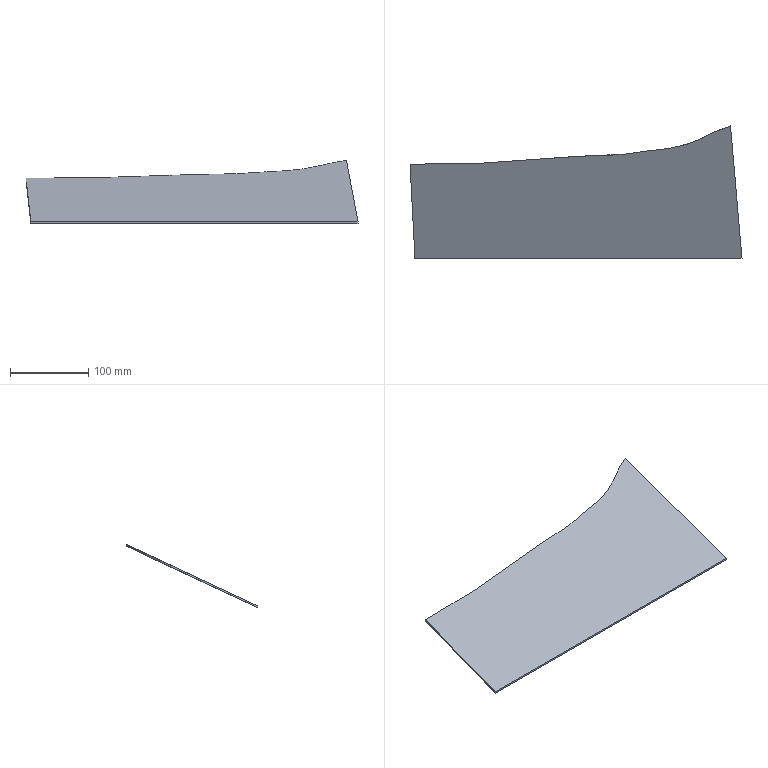Part | NX | features solid 2 | 1 solid | 6 faces | box 425.297 x 169.001 x 81.013 mm | volume 122184 mm3 | plane 5 | spline 1
STEP:
#1=CARTESIAN_POINT('',(239.735,-364.945,-0.306));
#2=VERTEX_POINT('',#1);
#3=CARTESIAN_POINT('',(246.027,-485.,-56.288));
#4=VERTEX_POINT('',#3);
#5=CARTESIAN_POINT('',(265.785,-861.995,-232.084));
#6=DIRECTION('',(0.04744,-0.9053,-0.4221));
#7=VECTOR('',#6,1000.);
#8=LINE('',#5,#7);
#9=EDGE_CURVE('',#2,#4,#8,.T.);
#10=ORIENTED_EDGE('',*,*,#9,.F.);
#11=CARTESIAN_POINT('',(239.735,-364.945,-2.513));
#12=VERTEX_POINT('',#11);
#13=CARTESIAN_POINT('',(239.735,-364.945,12.842));
#14=DIRECTION('',(0.,0.,-1.));
#15=VECTOR('',#14,1000.);
#16=LINE('',#13,#15);
#17=EDGE_CURVE('',#2,#12,#16,.T.);
#18=ORIENTED_EDGE('',*,*,#17,.T.);
#19=CARTESIAN_POINT('',(246.027,-485.,-58.495));
#20=VERTEX_POINT('',#19);
#21=CARTESIAN_POINT('',(265.74,-861.152,-233.898));
#22=DIRECTION('',(0.04744,-0.9053,-0.4221));
#23=VECTOR('',#22,1000.);
#24=LINE('',#21,#23);
#25=EDGE_CURVE('',#12,#20,#24,.T.);
#26=ORIENTED_EDGE('',*,*,#25,.T.);
#27=CARTESIAN_POINT('',(246.027,-485.,-75.));
#28=DIRECTION('',(0.,0.,1.));
#29=VECTOR('',#28,1000.);
#30=LINE('',#27,#29);
#31=EDGE_CURVE('',#4,#20,#30,.F.);
#32=ORIENTED_EDGE('',*,*,#31,.F.);
#33=EDGE_LOOP('',(#10,#18,#26,#32));
#34=FACE_BOUND('',#33,.T.);
#35=CARTESIAN_POINT('',(244.979,-465.,-85.));
#36=DIRECTION('',(-0.9986,-0.05234,0.));
#37=DIRECTION('',(0.05234,-0.9986,0.));
#38=AXIS2_PLACEMENT_3D('',#35,#36,#37);
#39=PLANE('',#38);
#40=ADVANCED_FACE('',(#34),#39,.T.);
#41=CARTESIAN_POINT('',(650.246,-315.999,22.518));
#42=VERTEX_POINT('',#41);
#43=CARTESIAN_POINT('',(650.246,-315.999,20.311));
#44=VERTEX_POINT('',#43);
#45=CARTESIAN_POINT('',(650.246,-315.999,25.721));
#46=DIRECTION('',(0.,0.,-1.));
#47=VECTOR('',#46,1000.);
#48=LINE('',#45,#47);
#49=EDGE_CURVE('',#42,#44,#48,.T.);
#50=ORIENTED_EDGE('',*,*,#49,.F.);
#51=CARTESIAN_POINT('',(665.032,-485.,-56.288));
#52=VERTEX_POINT('',#51);
#53=CARTESIAN_POINT('',(692.882,-803.329,-204.728));
#54=DIRECTION('',(-0.07904,0.9035,0.4213));
#55=VECTOR('',#54,1000.);
#56=LINE('',#53,#55);
#57=EDGE_CURVE('',#52,#42,#56,.T.);
#58=ORIENTED_EDGE('',*,*,#57,.F.);
#59=CARTESIAN_POINT('',(665.032,-485.,-58.495));
#60=VERTEX_POINT('',#59);
#61=CARTESIAN_POINT('',(665.032,-485.,-75.));
#62=DIRECTION('',(0.,0.,-1.));
#63=VECTOR('',#62,1000.);
#64=LINE('',#61,#63);
#65=EDGE_CURVE('',#60,#52,#64,.F.);
#66=ORIENTED_EDGE('',*,*,#65,.F.);
#67=CARTESIAN_POINT('',(692.809,-802.489,-206.543));
#68=DIRECTION('',(-0.07904,0.9035,0.4213));
#69=VECTOR('',#68,1000.);
#70=LINE('',#67,#69);
#71=EDGE_CURVE('',#60,#44,#70,.T.);
#72=ORIENTED_EDGE('',*,*,#71,.T.);
#73=EDGE_LOOP('',(#50,#58,#66,#72));
#74=FACE_BOUND('',#73,.T.);
#75=CARTESIAN_POINT('',(650.521,-319.136,95.148));
#76=DIRECTION('',(0.9962,0.08716,0.));
#77=DIRECTION('',(-0.08716,0.9962,0.));
#78=AXIS2_PLACEMENT_3D('',#75,#76,#77);
#79=PLANE('',#78);
#80=ADVANCED_FACE('',(#74),#79,.T.);
#81=CARTESIAN_POINT('',(-705.,-485.,-56.288));
#82=DIRECTION('',(-1.,0.,0.));
#83=VECTOR('',#82,1000.);
#84=LINE('',#81,#83);
#85=EDGE_CURVE('',#4,#52,#84,.F.);
#86=ORIENTED_EDGE('',*,*,#85,.F.);
#87=ORIENTED_EDGE('',*,*,#31,.T.);
#88=CARTESIAN_POINT('',(-705.,-485.,-58.495));
#89=DIRECTION('',(-1.,0.,0.));
#90=VECTOR('',#89,1000.);
#91=LINE('',#88,#90);
#92=EDGE_CURVE('',#20,#60,#91,.F.);
#93=ORIENTED_EDGE('',*,*,#92,.T.);
#94=ORIENTED_EDGE('',*,*,#65,.T.);
#95=EDGE_LOOP('',(#86,#87,#93,#94));
#96=FACE_BOUND('',#95,.T.);
#97=CARTESIAN_POINT('',(691.22,-485.,-75.));
#98=DIRECTION('',(0.,1.,0.));
#99=DIRECTION('',(-1.,0.,0.));
#100=AXIS2_PLACEMENT_3D('',#97,#98,#99);
#101=PLANE('',#100);
#102=ADVANCED_FACE('',(#96),#101,.F.);
#103=CARTESIAN_POINT('',(239.735,-364.945,-0.306));
#104=CARTESIAN_POINT('',(248.457,-364.848,-0.2607));
#105=CARTESIAN_POINT('',(261.539,-364.679,-0.1819));
#106=CARTESIAN_POINT('',(278.978,-364.377,-0.0408));
#107=CARTESIAN_POINT('',(292.052,-364.069,0.1028));
#108=CARTESIAN_POINT('',(305.133,-363.89,0.1863));
#109=CARTESIAN_POINT('',(318.228,-363.95,0.1583));
#110=CARTESIAN_POINT('',(331.306,-363.705,0.2723));
#111=CARTESIAN_POINT('',(344.341,-362.701,0.7406));
#112=CARTESIAN_POINT('',(357.365,-361.507,1.297));
#113=CARTESIAN_POINT('',(370.406,-360.618,1.712));
#114=CARTESIAN_POINT('',(383.445,-359.694,2.143));
#115=CARTESIAN_POINT('',(400.826,-358.378,2.756));
#116=CARTESIAN_POINT('',(422.546,-356.64,3.567));
#117=CARTESIAN_POINT('',(448.635,-354.979,4.341));
#118=CARTESIAN_POINT('',(470.408,-354.156,4.725));
#119=CARTESIAN_POINT('',(487.834,-353.633,4.969));
#120=CARTESIAN_POINT('',(500.903,-353.212,5.165));
#121=CARTESIAN_POINT('',(513.896,-352.294,5.593));
#122=CARTESIAN_POINT('',(526.75,-350.443,6.457));
#123=CARTESIAN_POINT('',(539.599,-348.555,7.337));
#124=CARTESIAN_POINT('',(552.484,-346.923,8.098));
#125=CARTESIAN_POINT('',(565.443,-345.75,8.645));
#126=CARTESIAN_POINT('',(578.275,-343.84,9.536));
#127=CARTESIAN_POINT('',(590.979,-340.657,11.02));
#128=CARTESIAN_POINT('',(603.227,-336.459,12.977));
#129=CARTESIAN_POINT('',(614.974,-331.322,15.373));
#130=CARTESIAN_POINT('',(626.223,-325.215,18.221));
#131=CARTESIAN_POINT('',(637.941,-320.005,20.65));
#132=CARTESIAN_POINT('',(646.238,-317.526,21.806));
#133=CARTESIAN_POINT('',(650.246,-315.999,22.518));
#134=B_SPLINE_CURVE_WITH_KNOTS('',3,(#103,#104,#105,#106,#107,#108,#109,#110,#111,#112,#113,#114,#115,#116,#117,#118,#119,#120,#121,#122,#123,#124,#125,#126,#127,#128,#129,#130,#131,#132,#133),.UNSPECIFIED.,.F.,.F.,(4,1,1,1,1,1,1,1,1,1,1,1,1,1,1,1,1,1,1,1,1,1,1,1,1,1,1,1,4),(0.9897,1.015,1.027,1.04,1.052,1.065,1.077,1.09,1.102,1.115,1.127,1.14,1.165,1.19,1.215,1.227,1.24,1.252,1.264,1.277,1.289,1.302,1.314,1.327,1.339,1.352,1.364,1.377,1.389),.UNSPECIFIED.);
#135=EDGE_CURVE('',#2,#42,#134,.T.);
#136=ORIENTED_EDGE('',*,*,#135,.F.);
#137=ORIENTED_EDGE('',*,*,#9,.T.);
#138=ORIENTED_EDGE('',*,*,#85,.T.);
#139=ORIENTED_EDGE('',*,*,#57,.T.);
#140=EDGE_LOOP('',(#136,#137,#138,#139));
#141=FACE_BOUND('',#140,.T.);
#142=CARTESIAN_POINT('',(-705.,-903.785,-251.571));
#143=DIRECTION('',(0.,-0.4226,0.9063));
#144=DIRECTION('',(1.,0.,0.));
#145=AXIS2_PLACEMENT_3D('',#142,#143,#144);
#146=PLANE('',#145);
#147=ADVANCED_FACE('',(#141),#146,.T.);
#148=ORIENTED_EDGE('',*,*,#25,.F.);
#149=CARTESIAN_POINT('',(239.735,-364.945,-2.513));
#150=CARTESIAN_POINT('',(248.405,-364.849,-2.468));
#151=CARTESIAN_POINT('',(261.41,-364.681,-2.39));
#152=CARTESIAN_POINT('',(278.749,-364.381,-2.25));
#153=CARTESIAN_POINT('',(291.751,-364.076,-2.107));
#154=CARTESIAN_POINT('',(304.755,-363.89,-2.021));
#155=CARTESIAN_POINT('',(317.764,-363.948,-2.048));
#156=CARTESIAN_POINT('',(330.768,-363.727,-1.945));
#157=CARTESIAN_POINT('',(343.759,-362.758,-1.493));
#158=CARTESIAN_POINT('',(356.746,-361.554,-0.9316));
#159=CARTESIAN_POINT('',(369.738,-360.664,-0.5162));
#160=CARTESIAN_POINT('',(382.73,-359.746,-0.0884));
#161=CARTESIAN_POINT('',(400.051,-358.44,0.5207));
#162=CARTESIAN_POINT('',(421.702,-356.703,1.33));
#163=CARTESIAN_POINT('',(447.685,-355.031,2.11));
#164=CARTESIAN_POINT('',(469.36,-354.188,2.504));
#165=CARTESIAN_POINT('',(486.728,-353.668,2.746));
#166=CARTESIAN_POINT('',(499.749,-353.253,2.939));
#167=CARTESIAN_POINT('',(512.717,-352.424,3.326));
#168=CARTESIAN_POINT('',(525.56,-350.628,4.164));
#169=CARTESIAN_POINT('',(538.388,-348.725,5.051));
#170=CARTESIAN_POINT('',(551.246,-347.056,5.829));
#171=CARTESIAN_POINT('',(564.17,-345.878,6.379));
#172=CARTESIAN_POINT('',(577.009,-344.08,7.217));
#173=CARTESIAN_POINT('',(589.7,-341.039,8.635));
#174=CARTESIAN_POINT('',(602.192,-336.862,10.582));
#175=CARTESIAN_POINT('',(614.217,-331.701,12.989));
#176=CARTESIAN_POINT('',(623.882,-326.499,15.415));
#177=CARTESIAN_POINT('',(631.764,-322.708,17.183));
#178=CARTESIAN_POINT('',(639.865,-319.452,18.701));
#179=CARTESIAN_POINT('',(646.165,-317.553,19.586));
#180=CARTESIAN_POINT('',(650.246,-315.999,20.311));
#181=B_SPLINE_CURVE_WITH_KNOTS('',3,(#149,#150,#151,#152,#153,#154,#155,#156,#157,#158,#159,#160,#161,#162,#163,#164,#165,#166,#167,#168,#169,#170,#171,#172,#173,#174,#175,#176,#177,#178,#179,#180),.UNSPECIFIED.,.F.,.F.,(4,1,1,1,1,1,1,1,1,1,1,1,1,1,1,1,1,1,1,1,1,1,1,1,1,1,1,1,1,4),(0.9451,0.9687,0.9805,0.9922,1.004,1.016,1.028,1.039,1.051,1.063,1.075,1.087,1.11,1.134,1.157,1.169,1.181,1.193,1.204,1.216,1.228,1.24,1.251,1.263,1.275,1.287,1.299,1.305,1.31,1.322),.UNSPECIFIED.);
#182=EDGE_CURVE('',#12,#44,#181,.T.);
#183=ORIENTED_EDGE('',*,*,#182,.T.);
#184=ORIENTED_EDGE('',*,*,#71,.F.);
#185=ORIENTED_EDGE('',*,*,#92,.F.);
#186=EDGE_LOOP('',(#148,#183,#184,#185));
#187=FACE_BOUND('',#186,.T.);
#188=CARTESIAN_POINT('',(-705.,-902.939,-253.384));
#189=DIRECTION('',(0.,-0.4226,0.9063));
#190=DIRECTION('',(1.,0.,0.));
#191=AXIS2_PLACEMENT_3D('',#188,#189,#190);
#192=PLANE('',#191);
#193=ADVANCED_FACE('',(#187),#192,.F.);
#194=ORIENTED_EDGE('',*,*,#17,.F.);
#195=ORIENTED_EDGE('',*,*,#135,.T.);
#196=ORIENTED_EDGE('',*,*,#49,.T.);
#197=ORIENTED_EDGE('',*,*,#182,.F.);
#198=EDGE_LOOP('',(#194,#195,#196,#197));
#199=FACE_BOUND('',#198,.T.);
#200=CARTESIAN_POINT('',(650.246,-315.999,22.668));
#201=CARTESIAN_POINT('',(650.246,-315.999,-2.663));
#202=CARTESIAN_POINT('',(646.189,-317.544,22.668));
#203=CARTESIAN_POINT('',(646.189,-317.544,-2.663));
#204=CARTESIAN_POINT('',(637.846,-320.029,22.668));
#205=CARTESIAN_POINT('',(637.846,-320.029,-2.663));
#206=CARTESIAN_POINT('',(625.95,-325.355,22.668));
#207=CARTESIAN_POINT('',(625.95,-325.355,-2.663));
#208=CARTESIAN_POINT('',(614.487,-331.574,22.668));
#209=CARTESIAN_POINT('',(614.487,-331.574,-2.663));
#210=CARTESIAN_POINT('',(602.518,-336.735,22.668));
#211=CARTESIAN_POINT('',(602.518,-336.735,-2.663));
#212=CARTESIAN_POINT('',(590.159,-340.902,22.668));
#213=CARTESIAN_POINT('',(590.159,-340.902,-2.663));
#214=CARTESIAN_POINT('',(577.496,-343.99,22.668));
#215=CARTESIAN_POINT('',(577.496,-343.99,-2.663));
#216=CARTESIAN_POINT('',(564.589,-345.838,22.668));
#217=CARTESIAN_POINT('',(564.589,-345.838,-2.663));
#218=CARTESIAN_POINT('',(551.614,-347.015,22.668));
#219=CARTESIAN_POINT('',(551.614,-347.015,-2.663));
#220=CARTESIAN_POINT('',(538.696,-348.681,22.668));
#221=CARTESIAN_POINT('',(538.696,-348.681,-2.663));
#222=CARTESIAN_POINT('',(525.807,-350.59,22.668));
#223=CARTESIAN_POINT('',(525.807,-350.59,-2.663));
#224=CARTESIAN_POINT('',(512.903,-352.405,22.668));
#225=CARTESIAN_POINT('',(512.903,-352.405,-2.663));
#226=CARTESIAN_POINT('',(499.902,-353.248,22.668));
#227=CARTESIAN_POINT('',(499.902,-353.248,-2.663));
#228=CARTESIAN_POINT('',(486.879,-353.663,22.668));
#229=CARTESIAN_POINT('',(486.879,-353.663,-2.663));
#230=CARTESIAN_POINT('',(469.52,-354.183,22.668));
#231=CARTESIAN_POINT('',(469.52,-354.183,-2.663));
#232=CARTESIAN_POINT('',(447.825,-355.023,22.668));
#233=CARTESIAN_POINT('',(447.825,-355.023,-2.663));
#234=CARTESIAN_POINT('',(421.824,-356.694,22.668));
#235=CARTESIAN_POINT('',(421.824,-356.694,-2.663));
#236=CARTESIAN_POINT('',(400.183,-358.429,22.668));
#237=CARTESIAN_POINT('',(400.183,-358.429,-2.663));
#238=CARTESIAN_POINT('',(382.864,-359.736,22.668));
#239=CARTESIAN_POINT('',(382.864,-359.736,-2.663));
#240=CARTESIAN_POINT('',(369.871,-360.655,22.668));
#241=CARTESIAN_POINT('',(369.871,-360.655,-2.663));
#242=CARTESIAN_POINT('',(356.875,-361.545,22.668));
#243=CARTESIAN_POINT('',(356.875,-361.545,-2.663));
#244=CARTESIAN_POINT('',(343.902,-362.744,22.668));
#245=CARTESIAN_POINT('',(343.902,-362.744,-2.663));
#246=CARTESIAN_POINT('',(330.912,-363.721,22.668));
#247=CARTESIAN_POINT('',(330.912,-363.721,-2.663));
#248=CARTESIAN_POINT('',(317.884,-363.949,22.668));
#249=CARTESIAN_POINT('',(317.884,-363.949,-2.663));
#250=CARTESIAN_POINT('',(304.858,-363.89,22.668));
#251=CARTESIAN_POINT('',(304.858,-363.89,-2.663));
#252=CARTESIAN_POINT('',(291.833,-364.074,22.668));
#253=CARTESIAN_POINT('',(291.833,-364.074,-2.663));
#254=CARTESIAN_POINT('',(278.81,-364.38,22.668));
#255=CARTESIAN_POINT('',(278.81,-364.38,-2.663));
#256=CARTESIAN_POINT('',(261.444,-364.68,22.668));
#257=CARTESIAN_POINT('',(261.444,-364.68,-2.663));
#258=CARTESIAN_POINT('',(248.419,-364.849,22.668));
#259=CARTESIAN_POINT('',(248.419,-364.849,-2.663));
#260=CARTESIAN_POINT('',(239.735,-364.945,22.668));
#261=CARTESIAN_POINT('',(239.735,-364.945,-2.663));
#262=B_SPLINE_SURFACE_WITH_KNOTS('',3,1,((#200,#201),(#202,#203),(#204,#205),(#206,#207),(#208,#209),(#210,#211),(#212,#213),(#214,#215),(#216,#217),(#218,#219),(#220,#221),(#222,#223),(#224,#225),(#226,#227),(#228,#229),(#230,#231),(#232,#233),(#234,#235),(#236,#237),(#238,#239),(#240,#241),(#242,#243),(#244,#245),(#246,#247),(#248,#249),(#250,#251),(#252,#253),(#254,#255),(#256,#257),(#258,#259),(#260,#261)),.SURF_OF_LINEAR_EXTRUSION.,.F.,.F.,.F.,(4,1,1,1,1,1,1,1,1,1,1,1,1,1,1,1,1,1,1,1,1,1,1,1,1,1,1,1,4),(2,2),(0.07339,0.07626,0.07912,0.08199,0.08485,0.08772,0.09058,0.09345,0.09631,0.09918,0.102,0.1049,0.1078,0.1106,0.1135,0.1192,0.125,0.1307,0.1336,0.1364,0.1393,0.1421,0.145,0.1479,0.1507,0.1536,0.1565,0.1593,0.1651),(0.,1.),.UNSPECIFIED.);
#263=ADVANCED_FACE('',(#199),#262,.F.);
#264=CLOSED_SHELL('',(#40,#80,#102,#147,#193,#263));
#265=MANIFOLD_SOLID_BREP('',#264);
#266=(LENGTH_UNIT()NAMED_UNIT(*)SI_UNIT(.MILLI.,.METRE.));
#267=UNCERTAINTY_MEASURE_WITH_UNIT(LENGTH_MEASURE(0.0508),#266,'','');
#268=(NAMED_UNIT(*)PLANE_ANGLE_UNIT()SI_UNIT($,.RADIAN.));
#269=(NAMED_UNIT(*)SI_UNIT($,.STERADIAN.)SOLID_ANGLE_UNIT());
#270=(GEOMETRIC_REPRESENTATION_CONTEXT(3)GLOBAL_UNCERTAINTY_ASSIGNED_CONTEXT((#267))GLOBAL_UNIT_ASSIGNED_CONTEXT((#266,#268,#269))REPRESENTATION_CONTEXT('',''));
#271=ADVANCED_BREP_SHAPE_REPRESENTATION('',(#265),#270);